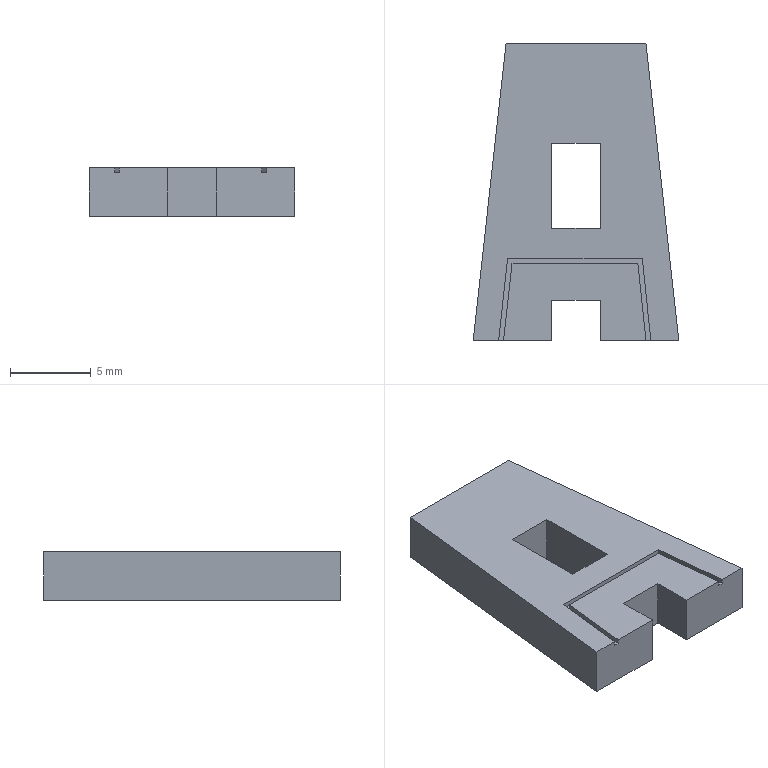Part | SolidWorks | features BaseBody 1 | 1 solid | 22 faces | box 12.712 x 18.351 x 3 mm | volume 516.696 mm3 | plane 21 | spline 1
STEP:
#1=CARTESIAN_POINT('',(103.606,-126.263,1.5));
#2=VERTEX_POINT('',#1);
#3=CARTESIAN_POINT('',(111.929,-126.263,1.5));
#4=VERTEX_POINT('',#3);
#5=CARTESIAN_POINT('',(103.606,-126.263,1.5));
#6=DIRECTION('',(1.,0.,0.));
#7=VECTOR('',#6,1000.);
#8=LINE('',#5,#7);
#9=EDGE_CURVE('',#2,#4,#8,.T.);
#10=ORIENTED_EDGE('',*,*,#9,.F.);
#11=CARTESIAN_POINT('',(103.606,-126.263,1.2));
#12=VERTEX_POINT('',#11);
#13=CARTESIAN_POINT('',(103.606,-126.263,1.2));
#14=DIRECTION('',(0.,0.,1.));
#15=VECTOR('',#14,1000.);
#16=LINE('',#13,#15);
#17=EDGE_CURVE('',#12,#2,#16,.T.);
#18=ORIENTED_EDGE('',*,*,#17,.F.);
#19=CARTESIAN_POINT('',(111.929,-126.263,1.2));
#20=VERTEX_POINT('',#19);
#21=CARTESIAN_POINT('',(103.606,-126.263,1.2));
#22=DIRECTION('',(1.,0.,0.));
#23=VECTOR('',#22,1000.);
#24=LINE('',#21,#23);
#25=EDGE_CURVE('',#12,#20,#24,.T.);
#26=ORIENTED_EDGE('',*,*,#25,.T.);
#27=CARTESIAN_POINT('',(111.929,-126.263,1.2));
#28=DIRECTION('',(0.,0.,1.));
#29=VECTOR('',#28,1000.);
#30=LINE('',#27,#29);
#31=EDGE_CURVE('',#20,#4,#30,.T.);
#32=ORIENTED_EDGE('',*,*,#31,.T.);
#33=EDGE_LOOP('',(#10,#18,#26,#32));
#34=FACE_OUTER_BOUND('',#33,.T.);
#35=CARTESIAN_POINT('',(103.606,-126.263,1.2));
#36=DIRECTION('',(0.,-1.,0.));
#37=DIRECTION('',(0.,0.,-1.));
#38=AXIS2_PLACEMENT_3D('',#35,#36,#37);
#39=PLANE('',#38);
#40=ADVANCED_FACE('',(#34),#39,.T.);
#41=CARTESIAN_POINT('',(103.875,-126.563,1.5));
#42=VERTEX_POINT('',#41);
#43=CARTESIAN_POINT('',(111.659,-126.563,1.5));
#44=VERTEX_POINT('',#43);
#45=CARTESIAN_POINT('',(103.606,-126.563,1.5));
#46=DIRECTION('',(1.,0.,0.));
#47=VECTOR('',#46,1000.);
#48=LINE('',#45,#47);
#49=EDGE_CURVE('',#42,#44,#48,.T.);
#50=ORIENTED_EDGE('',*,*,#49,.T.);
#51=CARTESIAN_POINT('',(111.659,-126.563,1.2));
#52=VERTEX_POINT('',#51);
#53=CARTESIAN_POINT('',(111.659,-126.563,1.2));
#54=DIRECTION('',(0.,0.,1.));
#55=VECTOR('',#54,1000.);
#56=LINE('',#53,#55);
#57=EDGE_CURVE('',#52,#44,#56,.T.);
#58=ORIENTED_EDGE('',*,*,#57,.F.);
#59=CARTESIAN_POINT('',(103.875,-126.563,1.2));
#60=VERTEX_POINT('',#59);
#61=CARTESIAN_POINT('',(103.606,-126.563,1.2));
#62=DIRECTION('',(1.,0.,0.));
#63=VECTOR('',#62,1000.);
#64=LINE('',#61,#63);
#65=EDGE_CURVE('',#60,#52,#64,.T.);
#66=ORIENTED_EDGE('',*,*,#65,.F.);
#67=CARTESIAN_POINT('',(103.875,-126.563,1.2));
#68=DIRECTION('',(0.,0.,1.));
#69=VECTOR('',#68,1000.);
#70=LINE('',#67,#69);
#71=EDGE_CURVE('',#60,#42,#70,.T.);
#72=ORIENTED_EDGE('',*,*,#71,.T.);
#73=EDGE_LOOP('',(#50,#58,#66,#72));
#74=FACE_OUTER_BOUND('',#73,.T.);
#75=CARTESIAN_POINT('',(103.606,-126.563,1.2));
#76=DIRECTION('',(0.,-1.,0.));
#77=DIRECTION('',(0.,0.,-1.));
#78=AXIS2_PLACEMENT_3D('',#75,#76,#77);
#79=PLANE('',#78);
#80=ADVANCED_FACE('',(#74),#79,.F.);
#81=CARTESIAN_POINT('',(112.461,-131.327,1.2));
#82=VERTEX_POINT('',#81);
#83=CARTESIAN_POINT('',(112.461,-131.327,1.5));
#84=VERTEX_POINT('',#83);
#85=CARTESIAN_POINT('',(112.461,-131.327,-1.5));
#86=DIRECTION('',(0.,0.,1.));
#87=VECTOR('',#86,1000.);
#88=LINE('',#85,#87);
#89=EDGE_CURVE('',#82,#84,#88,.T.);
#90=ORIENTED_EDGE('',*,*,#89,.T.);
#91=CARTESIAN_POINT('',(111.929,-126.263,1.5));
#92=DIRECTION('',(0.1043,-0.9945,0.));
#93=VECTOR('',#92,1000.);
#94=LINE('',#91,#93);
#95=EDGE_CURVE('',#4,#84,#94,.T.);
#96=ORIENTED_EDGE('',*,*,#95,.F.);
#97=ORIENTED_EDGE('',*,*,#31,.F.);
#98=CARTESIAN_POINT('',(111.929,-126.263,1.2));
#99=DIRECTION('',(0.1043,-0.9945,0.));
#100=VECTOR('',#99,1000.);
#101=LINE('',#98,#100);
#102=EDGE_CURVE('',#20,#82,#101,.T.);
#103=ORIENTED_EDGE('',*,*,#102,.T.);
#104=EDGE_LOOP('',(#90,#96,#97,#103));
#105=FACE_OUTER_BOUND('',#104,.T.);
#106=CARTESIAN_POINT('',(111.929,-126.263,1.2));
#107=DIRECTION('',(-0.9945,-0.1043,0.));
#108=DIRECTION('',(-0.1043,0.9945,0.));
#109=AXIS2_PLACEMENT_3D('',#106,#107,#108);
#110=PLANE('',#109);
#111=ADVANCED_FACE('',(#105),#110,.T.);
#112=CARTESIAN_POINT('',(103.046,-131.327,1.5));
#113=VERTEX_POINT('',#112);
#114=CARTESIAN_POINT('',(103.046,-131.327,1.2));
#115=VERTEX_POINT('',#114);
#116=CARTESIAN_POINT('',(103.046,-131.327,-1.5));
#117=DIRECTION('',(0.,0.,-1.));
#118=VECTOR('',#117,1000.);
#119=LINE('',#116,#118);
#120=EDGE_CURVE('',#113,#115,#119,.T.);
#121=ORIENTED_EDGE('',*,*,#120,.T.);
#122=CARTESIAN_POINT('',(102.875,-132.867,1.2));
#123=DIRECTION('',(0.1101,0.9939,0.));
#124=VECTOR('',#123,1000.);
#125=LINE('',#122,#124);
#126=EDGE_CURVE('',#115,#12,#125,.T.);
#127=ORIENTED_EDGE('',*,*,#126,.T.);
#128=ORIENTED_EDGE('',*,*,#17,.T.);
#129=CARTESIAN_POINT('',(116.164,-12.864,1.5));
#130=DIRECTION('',(0.1101,0.9939,0.));
#131=VECTOR('',#130,1000.);
#132=LINE('',#129,#131);
#133=EDGE_CURVE('',#113,#2,#132,.T.);
#134=ORIENTED_EDGE('',*,*,#133,.F.);
#135=EDGE_LOOP('',(#121,#127,#128,#134));
#136=FACE_OUTER_BOUND('',#135,.T.);
#137=CARTESIAN_POINT('',(102.875,-132.867,1.2));
#138=DIRECTION('',(0.9939,-0.1101,0.));
#139=DIRECTION('',(0.,0.,-1.));
#140=AXIS2_PLACEMENT_3D('',#137,#138,#139);
#141=PLANE('',#140);
#142=ADVANCED_FACE('',(#136),#141,.T.);
#143=CARTESIAN_POINT('',(103.347,-131.327,1.5));
#144=VERTEX_POINT('',#143);
#145=CARTESIAN_POINT('',(116.462,-12.897,1.5));
#146=DIRECTION('',(0.1101,0.9939,0.));
#147=VECTOR('',#146,1000.);
#148=LINE('',#145,#147);
#149=EDGE_CURVE('',#144,#42,#148,.T.);
#150=ORIENTED_EDGE('',*,*,#149,.T.);
#151=ORIENTED_EDGE('',*,*,#71,.F.);
#152=CARTESIAN_POINT('',(103.347,-131.327,1.2));
#153=VERTEX_POINT('',#152);
#154=CARTESIAN_POINT('',(103.173,-132.9,1.2));
#155=DIRECTION('',(0.1101,0.9939,0.));
#156=VECTOR('',#155,1000.);
#157=LINE('',#154,#156);
#158=EDGE_CURVE('',#153,#60,#157,.T.);
#159=ORIENTED_EDGE('',*,*,#158,.F.);
#160=CARTESIAN_POINT('',(103.347,-131.327,-1.5));
#161=DIRECTION('',(0.,0.,-1.));
#162=VECTOR('',#161,1000.);
#163=LINE('',#160,#162);
#164=EDGE_CURVE('',#144,#153,#163,.T.);
#165=ORIENTED_EDGE('',*,*,#164,.F.);
#166=EDGE_LOOP('',(#150,#151,#159,#165));
#167=FACE_OUTER_BOUND('',#166,.T.);
#168=CARTESIAN_POINT('',(103.173,-132.9,1.2));
#169=DIRECTION('',(0.9939,-0.1101,0.));
#170=DIRECTION('',(0.,0.,-1.));
#171=AXIS2_PLACEMENT_3D('',#168,#169,#170);
#172=PLANE('',#171);
#173=ADVANCED_FACE('',(#167),#172,.F.);
#174=CARTESIAN_POINT('',(112.159,-131.327,1.2));
#175=VERTEX_POINT('',#174);
#176=CARTESIAN_POINT('',(111.631,-126.294,1.2));
#177=DIRECTION('',(0.1043,-0.9945,0.));
#178=VECTOR('',#177,1000.);
#179=LINE('',#176,#178);
#180=EDGE_CURVE('',#52,#175,#179,.T.);
#181=ORIENTED_EDGE('',*,*,#180,.F.);
#182=ORIENTED_EDGE('',*,*,#57,.T.);
#183=CARTESIAN_POINT('',(112.159,-131.327,1.5));
#184=VERTEX_POINT('',#183);
#185=CARTESIAN_POINT('',(111.631,-126.294,1.5));
#186=DIRECTION('',(0.1043,-0.9945,0.));
#187=VECTOR('',#186,1000.);
#188=LINE('',#185,#187);
#189=EDGE_CURVE('',#44,#184,#188,.T.);
#190=ORIENTED_EDGE('',*,*,#189,.T.);
#191=CARTESIAN_POINT('',(112.159,-131.327,-1.5));
#192=DIRECTION('',(0.,0.,1.));
#193=VECTOR('',#192,1000.);
#194=LINE('',#191,#193);
#195=EDGE_CURVE('',#175,#184,#194,.T.);
#196=ORIENTED_EDGE('',*,*,#195,.F.);
#197=EDGE_LOOP('',(#181,#182,#190,#196));
#198=FACE_OUTER_BOUND('',#197,.T.);
#199=CARTESIAN_POINT('',(111.631,-126.294,1.2));
#200=DIRECTION('',(-0.9945,-0.1043,0.));
#201=DIRECTION('',(-0.1043,0.9945,0.));
#202=AXIS2_PLACEMENT_3D('',#199,#200,#201);
#203=PLANE('',#202);
#204=ADVANCED_FACE('',(#198),#203,.F.);
#205=ORIENTED_EDGE('',*,*,#102,.F.);
#206=ORIENTED_EDGE('',*,*,#25,.F.);
#207=ORIENTED_EDGE('',*,*,#126,.F.);
#208=CARTESIAN_POINT('',(0.,-131.327,1.2));
#209=DIRECTION('',(-1.,0.,0.));
#210=VECTOR('',#209,1000.);
#211=LINE('',#208,#210);
#212=EDGE_CURVE('',#153,#115,#211,.T.);
#213=ORIENTED_EDGE('',*,*,#212,.F.);
#214=ORIENTED_EDGE('',*,*,#158,.T.);
#215=ORIENTED_EDGE('',*,*,#65,.T.);
#216=ORIENTED_EDGE('',*,*,#180,.T.);
#217=CARTESIAN_POINT('',(0.,-131.327,1.2));
#218=DIRECTION('',(-1.,0.,0.));
#219=VECTOR('',#218,1000.);
#220=LINE('',#217,#219);
#221=EDGE_CURVE('',#82,#175,#220,.T.);
#222=ORIENTED_EDGE('',*,*,#221,.F.);
#223=EDGE_LOOP('',(#205,#206,#207,#213,#214,#215,#216,#222));
#224=FACE_OUTER_BOUND('',#223,.T.);
#225=CARTESIAN_POINT('',(0.,0.,1.2));
#226=DIRECTION('',(0.,0.,-1.));
#227=DIRECTION('',(0.,-1.,0.));
#228=AXIS2_PLACEMENT_3D('',#225,#226,#227);
#229=PLANE('',#228);
#230=ADVANCED_FACE('',(#224),#229,.F.);
#231=ORIENTED_EDGE('',*,*,#189,.F.);
#232=ORIENTED_EDGE('',*,*,#49,.F.);
#233=ORIENTED_EDGE('',*,*,#149,.F.);
#234=CARTESIAN_POINT('',(106.335,-131.327,1.5));
#235=VERTEX_POINT('',#234);
#236=CARTESIAN_POINT('',(0.,-131.327,1.5));
#237=DIRECTION('',(-1.,0.,0.));
#238=VECTOR('',#237,1000.);
#239=LINE('',#236,#238);
#240=EDGE_CURVE('',#235,#144,#239,.T.);
#241=ORIENTED_EDGE('',*,*,#240,.F.);
#242=CARTESIAN_POINT('',(106.335,-128.839,1.5));
#243=VERTEX_POINT('',#242);
#244=CARTESIAN_POINT('',(106.335,0.,1.5));
#245=DIRECTION('',(0.,-1.,0.));
#246=VECTOR('',#245,1000.);
#247=LINE('',#244,#246);
#248=EDGE_CURVE('',#243,#235,#247,.T.);
#249=ORIENTED_EDGE('',*,*,#248,.F.);
#250=CARTESIAN_POINT('',(109.33,-128.839,1.5));
#251=VERTEX_POINT('',#250);
#252=CARTESIAN_POINT('',(0.,-128.839,1.5));
#253=DIRECTION('',(-1.,0.,0.));
#254=VECTOR('',#253,1000.);
#255=LINE('',#252,#254);
#256=EDGE_CURVE('',#251,#243,#255,.T.);
#257=ORIENTED_EDGE('',*,*,#256,.F.);
#258=CARTESIAN_POINT('',(109.33,-131.327,1.5));
#259=VERTEX_POINT('',#258);
#260=CARTESIAN_POINT('',(109.33,0.,1.5));
#261=DIRECTION('',(0.,1.,0.));
#262=VECTOR('',#261,1000.);
#263=LINE('',#260,#262);
#264=EDGE_CURVE('',#259,#251,#263,.T.);
#265=ORIENTED_EDGE('',*,*,#264,.F.);
#266=CARTESIAN_POINT('',(0.,-131.327,1.5));
#267=DIRECTION('',(-1.,0.,0.));
#268=VECTOR('',#267,1000.);
#269=LINE('',#266,#268);
#270=EDGE_CURVE('',#184,#259,#269,.T.);
#271=ORIENTED_EDGE('',*,*,#270,.F.);
#272=EDGE_LOOP('',(#231,#232,#233,#241,#249,#257,#265,#271));
#273=FACE_OUTER_BOUND('',#272,.T.);
#274=CARTESIAN_POINT('',(0.,0.,1.5));
#275=DIRECTION('',(0.,0.,1.));
#276=DIRECTION('',(1.,0.,0.));
#277=AXIS2_PLACEMENT_3D('',#274,#275,#276);
#278=PLANE('',#277);
#279=ADVANCED_FACE('',(#273),#278,.T.);
#280=CARTESIAN_POINT('',(106.335,-119.133,-1.5));
#281=VERTEX_POINT('',#280);
#282=CARTESIAN_POINT('',(106.335,-124.395,-1.5));
#283=VERTEX_POINT('',#282);
#284=CARTESIAN_POINT('',(106.335,0.,-1.5));
#285=DIRECTION('',(0.,-1.,0.));
#286=VECTOR('',#285,1000.);
#287=LINE('',#284,#286);
#288=EDGE_CURVE('',#281,#283,#287,.T.);
#289=ORIENTED_EDGE('',*,*,#288,.T.);
#290=CARTESIAN_POINT('',(109.33,-124.395,-1.5));
#291=VERTEX_POINT('',#290);
#292=CARTESIAN_POINT('',(0.,-124.395,-1.5));
#293=DIRECTION('',(1.,0.,0.));
#294=VECTOR('',#293,1000.);
#295=LINE('',#292,#294);
#296=EDGE_CURVE('',#283,#291,#295,.T.);
#297=ORIENTED_EDGE('',*,*,#296,.T.);
#298=CARTESIAN_POINT('',(109.33,-119.133,-1.5));
#299=VERTEX_POINT('',#298);
#300=CARTESIAN_POINT('',(109.33,0.,-1.5));
#301=DIRECTION('',(0.,1.,0.));
#302=VECTOR('',#301,1000.);
#303=LINE('',#300,#302);
#304=EDGE_CURVE('',#291,#299,#303,.T.);
#305=ORIENTED_EDGE('',*,*,#304,.T.);
#306=CARTESIAN_POINT('',(0.,-119.133,-1.5));
#307=DIRECTION('',(-1.,0.,0.));
#308=VECTOR('',#307,1000.);
#309=LINE('',#306,#308);
#310=EDGE_CURVE('',#299,#281,#309,.T.);
#311=ORIENTED_EDGE('',*,*,#310,.T.);
#312=EDGE_LOOP('',(#289,#297,#305,#311));
#313=FACE_BOUND('',#312,.T.);
#314=CARTESIAN_POINT('',(101.476,-131.327,-1.5));
#315=VERTEX_POINT('',#314);
#316=CARTESIAN_POINT('',(103.509,-112.976,-1.5));
#317=VERTEX_POINT('',#316);
#318=CARTESIAN_POINT('',(101.476,-131.327,-1.5));
#319=CARTESIAN_POINT('',(102.154,-125.21,-1.5));
#320=CARTESIAN_POINT('',(102.831,-119.094,-1.5));
#321=CARTESIAN_POINT('',(103.509,-112.976,-1.5));
#322=B_SPLINE_CURVE_WITH_KNOTS('',3,(#318,#319,#320,#321),.UNSPECIFIED.,.F.,.F.,(4,4),(0.06667,0.1333),.UNSPECIFIED.);
#323=EDGE_CURVE('',#315,#317,#322,.T.);
#324=ORIENTED_EDGE('',*,*,#323,.T.);
#325=CARTESIAN_POINT('',(112.156,-112.976,-1.5));
#326=VERTEX_POINT('',#325);
#327=CARTESIAN_POINT('',(0.,-112.976,-1.5));
#328=DIRECTION('',(1.,0.,0.));
#329=VECTOR('',#328,1000.);
#330=LINE('',#327,#329);
#331=EDGE_CURVE('',#317,#326,#330,.T.);
#332=ORIENTED_EDGE('',*,*,#331,.T.);
#333=CARTESIAN_POINT('',(114.188,-131.327,-1.5));
#334=VERTEX_POINT('',#333);
#335=CARTESIAN_POINT('',(98.438,10.901,-1.5));
#336=DIRECTION('',(0.1101,-0.9939,0.));
#337=VECTOR('',#336,1000.);
#338=LINE('',#335,#337);
#339=EDGE_CURVE('',#326,#334,#338,.T.);
#340=ORIENTED_EDGE('',*,*,#339,.T.);
#341=CARTESIAN_POINT('',(109.33,-131.327,-1.5));
#342=VERTEX_POINT('',#341);
#343=CARTESIAN_POINT('',(0.,-131.327,-1.5));
#344=DIRECTION('',(-1.,0.,0.));
#345=VECTOR('',#344,1000.);
#346=LINE('',#343,#345);
#347=EDGE_CURVE('',#334,#342,#346,.T.);
#348=ORIENTED_EDGE('',*,*,#347,.T.);
#349=CARTESIAN_POINT('',(109.33,-128.839,-1.5));
#350=VERTEX_POINT('',#349);
#351=CARTESIAN_POINT('',(109.33,0.,-1.5));
#352=DIRECTION('',(0.,1.,0.));
#353=VECTOR('',#352,1000.);
#354=LINE('',#351,#353);
#355=EDGE_CURVE('',#342,#350,#354,.T.);
#356=ORIENTED_EDGE('',*,*,#355,.T.);
#357=CARTESIAN_POINT('',(106.335,-128.839,-1.5));
#358=VERTEX_POINT('',#357);
#359=CARTESIAN_POINT('',(0.,-128.839,-1.5));
#360=DIRECTION('',(-1.,0.,0.));
#361=VECTOR('',#360,1000.);
#362=LINE('',#359,#361);
#363=EDGE_CURVE('',#350,#358,#362,.T.);
#364=ORIENTED_EDGE('',*,*,#363,.T.);
#365=CARTESIAN_POINT('',(106.335,-131.327,-1.5));
#366=VERTEX_POINT('',#365);
#367=CARTESIAN_POINT('',(106.335,0.,-1.5));
#368=DIRECTION('',(0.,-1.,0.));
#369=VECTOR('',#368,1000.);
#370=LINE('',#367,#369);
#371=EDGE_CURVE('',#358,#366,#370,.T.);
#372=ORIENTED_EDGE('',*,*,#371,.T.);
#373=CARTESIAN_POINT('',(0.,-131.327,-1.5));
#374=DIRECTION('',(-1.,0.,0.));
#375=VECTOR('',#374,1000.);
#376=LINE('',#373,#375);
#377=EDGE_CURVE('',#366,#315,#376,.T.);
#378=ORIENTED_EDGE('',*,*,#377,.T.);
#379=EDGE_LOOP('',(#324,#332,#340,#348,#356,#364,#372,#378));
#380=FACE_OUTER_BOUND('',#379,.T.);
#381=CARTESIAN_POINT('',(0.,0.,-1.5));
#382=DIRECTION('',(0.,0.,1.));
#383=DIRECTION('',(1.,0.,0.));
#384=AXIS2_PLACEMENT_3D('',#381,#382,#383);
#385=PLANE('',#384);
#386=ADVANCED_FACE('',(#313,#380),#385,.F.);
#387=CARTESIAN_POINT('',(109.33,-119.133,1.5));
#388=VERTEX_POINT('',#387);
#389=CARTESIAN_POINT('',(106.335,-119.133,1.5));
#390=VERTEX_POINT('',#389);
#391=CARTESIAN_POINT('',(0.,-119.133,1.5));
#392=DIRECTION('',(-1.,0.,0.));
#393=VECTOR('',#392,1000.);
#394=LINE('',#391,#393);
#395=EDGE_CURVE('',#388,#390,#394,.T.);
#396=ORIENTED_EDGE('',*,*,#395,.T.);
#397=CARTESIAN_POINT('',(106.335,-119.133,-1.5));
#398=DIRECTION('',(0.,0.,1.));
#399=VECTOR('',#398,1000.);
#400=LINE('',#397,#399);
#401=EDGE_CURVE('',#281,#390,#400,.T.);
#402=ORIENTED_EDGE('',*,*,#401,.F.);
#403=ORIENTED_EDGE('',*,*,#310,.F.);
#404=CARTESIAN_POINT('',(109.33,-119.133,-1.5));
#405=DIRECTION('',(0.,0.,1.));
#406=VECTOR('',#405,1000.);
#407=LINE('',#404,#406);
#408=EDGE_CURVE('',#299,#388,#407,.T.);
#409=ORIENTED_EDGE('',*,*,#408,.T.);
#410=EDGE_LOOP('',(#396,#402,#403,#409));
#411=FACE_OUTER_BOUND('',#410,.T.);
#412=CARTESIAN_POINT('',(0.,-119.133,-1.5));
#413=DIRECTION('',(0.,1.,0.));
#414=DIRECTION('',(1.,0.,0.));
#415=AXIS2_PLACEMENT_3D('',#412,#413,#414);
#416=PLANE('',#415);
#417=ADVANCED_FACE('',(#411),#416,.F.);
#418=ORIENTED_EDGE('',*,*,#240,.T.);
#419=ORIENTED_EDGE('',*,*,#164,.T.);
#420=ORIENTED_EDGE('',*,*,#212,.T.);
#421=ORIENTED_EDGE('',*,*,#120,.F.);
#422=CARTESIAN_POINT('',(101.476,-131.327,1.5));
#423=VERTEX_POINT('',#422);
#424=CARTESIAN_POINT('',(0.,-131.327,1.5));
#425=DIRECTION('',(-1.,0.,0.));
#426=VECTOR('',#425,1000.);
#427=LINE('',#424,#426);
#428=EDGE_CURVE('',#113,#423,#427,.T.);
#429=ORIENTED_EDGE('',*,*,#428,.T.);
#430=CARTESIAN_POINT('',(101.476,-131.327,-1.5));
#431=DIRECTION('',(0.,0.,1.));
#432=VECTOR('',#431,1000.);
#433=LINE('',#430,#432);
#434=EDGE_CURVE('',#315,#423,#433,.T.);
#435=ORIENTED_EDGE('',*,*,#434,.F.);
#436=ORIENTED_EDGE('',*,*,#377,.F.);
#437=CARTESIAN_POINT('',(106.335,-131.327,-1.5));
#438=DIRECTION('',(0.,0.,1.));
#439=VECTOR('',#438,1000.);
#440=LINE('',#437,#439);
#441=EDGE_CURVE('',#366,#235,#440,.T.);
#442=ORIENTED_EDGE('',*,*,#441,.T.);
#443=EDGE_LOOP('',(#418,#419,#420,#421,#429,#435,#436,#442));
#444=FACE_OUTER_BOUND('',#443,.T.);
#445=CARTESIAN_POINT('',(0.,-131.327,-1.5));
#446=DIRECTION('',(0.,1.,0.));
#447=DIRECTION('',(1.,0.,0.));
#448=AXIS2_PLACEMENT_3D('',#445,#446,#447);
#449=PLANE('',#448);
#450=ADVANCED_FACE('',(#444),#449,.F.);
#451=ORIENTED_EDGE('',*,*,#248,.T.);
#452=ORIENTED_EDGE('',*,*,#441,.F.);
#453=ORIENTED_EDGE('',*,*,#371,.F.);
#454=CARTESIAN_POINT('',(106.335,-128.839,-1.5));
#455=DIRECTION('',(0.,0.,1.));
#456=VECTOR('',#455,1000.);
#457=LINE('',#454,#456);
#458=EDGE_CURVE('',#358,#243,#457,.T.);
#459=ORIENTED_EDGE('',*,*,#458,.T.);
#460=EDGE_LOOP('',(#451,#452,#453,#459));
#461=FACE_OUTER_BOUND('',#460,.T.);
#462=CARTESIAN_POINT('',(106.335,0.,-1.5));
#463=DIRECTION('',(-1.,0.,0.));
#464=DIRECTION('',(0.,0.,1.));
#465=AXIS2_PLACEMENT_3D('',#462,#463,#464);
#466=PLANE('',#465);
#467=ADVANCED_FACE('',(#461),#466,.F.);
#468=ORIENTED_EDGE('',*,*,#256,.T.);
#469=ORIENTED_EDGE('',*,*,#458,.F.);
#470=ORIENTED_EDGE('',*,*,#363,.F.);
#471=CARTESIAN_POINT('',(109.33,-128.839,-1.5));
#472=DIRECTION('',(0.,0.,1.));
#473=VECTOR('',#472,1000.);
#474=LINE('',#471,#473);
#475=EDGE_CURVE('',#350,#251,#474,.T.);
#476=ORIENTED_EDGE('',*,*,#475,.T.);
#477=EDGE_LOOP('',(#468,#469,#470,#476));
#478=FACE_OUTER_BOUND('',#477,.T.);
#479=CARTESIAN_POINT('',(0.,-128.839,-1.5));
#480=DIRECTION('',(0.,1.,0.));
#481=DIRECTION('',(1.,0.,0.));
#482=AXIS2_PLACEMENT_3D('',#479,#480,#481);
#483=PLANE('',#482);
#484=ADVANCED_FACE('',(#478),#483,.F.);
#485=ORIENTED_EDGE('',*,*,#264,.T.);
#486=ORIENTED_EDGE('',*,*,#475,.F.);
#487=ORIENTED_EDGE('',*,*,#355,.F.);
#488=CARTESIAN_POINT('',(109.33,-131.327,-1.5));
#489=DIRECTION('',(0.,0.,1.));
#490=VECTOR('',#489,1000.);
#491=LINE('',#488,#490);
#492=EDGE_CURVE('',#342,#259,#491,.T.);
#493=ORIENTED_EDGE('',*,*,#492,.T.);
#494=EDGE_LOOP('',(#485,#486,#487,#493));
#495=FACE_OUTER_BOUND('',#494,.T.);
#496=CARTESIAN_POINT('',(109.33,0.,-1.5));
#497=DIRECTION('',(1.,0.,0.));
#498=DIRECTION('',(0.,1.,0.));
#499=AXIS2_PLACEMENT_3D('',#496,#497,#498);
#500=PLANE('',#499);
#501=ADVANCED_FACE('',(#495),#500,.F.);
#502=ORIENTED_EDGE('',*,*,#221,.T.);
#503=ORIENTED_EDGE('',*,*,#195,.T.);
#504=ORIENTED_EDGE('',*,*,#270,.T.);
#505=ORIENTED_EDGE('',*,*,#492,.F.);
#506=ORIENTED_EDGE('',*,*,#347,.F.);
#507=CARTESIAN_POINT('',(114.188,-131.327,1.5));
#508=VERTEX_POINT('',#507);
#509=CARTESIAN_POINT('',(114.188,-131.327,-1.5));
#510=DIRECTION('',(0.,0.,1.));
#511=VECTOR('',#510,1000.);
#512=LINE('',#509,#511);
#513=EDGE_CURVE('',#334,#508,#512,.T.);
#514=ORIENTED_EDGE('',*,*,#513,.T.);
#515=CARTESIAN_POINT('',(0.,-131.327,1.5));
#516=DIRECTION('',(-1.,0.,0.));
#517=VECTOR('',#516,1000.);
#518=LINE('',#515,#517);
#519=EDGE_CURVE('',#508,#84,#518,.T.);
#520=ORIENTED_EDGE('',*,*,#519,.T.);
#521=ORIENTED_EDGE('',*,*,#89,.F.);
#522=EDGE_LOOP('',(#502,#503,#504,#505,#506,#514,#520,#521));
#523=FACE_OUTER_BOUND('',#522,.T.);
#524=CARTESIAN_POINT('',(0.,-131.327,-1.5));
#525=DIRECTION('',(0.,1.,0.));
#526=DIRECTION('',(1.,0.,0.));
#527=AXIS2_PLACEMENT_3D('',#524,#525,#526);
#528=PLANE('',#527);
#529=ADVANCED_FACE('',(#523),#528,.F.);
#530=CARTESIAN_POINT('',(112.156,-112.976,1.5));
#531=VERTEX_POINT('',#530);
#532=CARTESIAN_POINT('',(98.438,10.901,1.5));
#533=DIRECTION('',(0.1101,-0.9939,0.));
#534=VECTOR('',#533,1000.);
#535=LINE('',#532,#534);
#536=EDGE_CURVE('',#531,#508,#535,.T.);
#537=ORIENTED_EDGE('',*,*,#536,.T.);
#538=ORIENTED_EDGE('',*,*,#513,.F.);
#539=ORIENTED_EDGE('',*,*,#339,.F.);
#540=CARTESIAN_POINT('',(112.156,-112.976,-1.5));
#541=DIRECTION('',(0.,0.,1.));
#542=VECTOR('',#541,1000.);
#543=LINE('',#540,#542);
#544=EDGE_CURVE('',#326,#531,#543,.T.);
#545=ORIENTED_EDGE('',*,*,#544,.T.);
#546=EDGE_LOOP('',(#537,#538,#539,#545));
#547=FACE_OUTER_BOUND('',#546,.T.);
#548=CARTESIAN_POINT('',(98.438,10.901,-1.5));
#549=DIRECTION('',(-0.9939,-0.1101,0.));
#550=DIRECTION('',(-0.1101,0.9939,0.));
#551=AXIS2_PLACEMENT_3D('',#548,#549,#550);
#552=PLANE('',#551);
#553=ADVANCED_FACE('',(#547),#552,.F.);
#554=CARTESIAN_POINT('',(103.509,-112.976,1.5));
#555=VERTEX_POINT('',#554);
#556=CARTESIAN_POINT('',(0.,-112.976,1.5));
#557=DIRECTION('',(1.,0.,0.));
#558=VECTOR('',#557,1000.);
#559=LINE('',#556,#558);
#560=EDGE_CURVE('',#555,#531,#559,.T.);
#561=ORIENTED_EDGE('',*,*,#560,.T.);
#562=ORIENTED_EDGE('',*,*,#544,.F.);
#563=ORIENTED_EDGE('',*,*,#331,.F.);
#564=CARTESIAN_POINT('',(103.509,-112.976,-1.5));
#565=DIRECTION('',(0.,0.,1.));
#566=VECTOR('',#565,1000.);
#567=LINE('',#564,#566);
#568=EDGE_CURVE('',#317,#555,#567,.T.);
#569=ORIENTED_EDGE('',*,*,#568,.T.);
#570=EDGE_LOOP('',(#561,#562,#563,#569));
#571=FACE_OUTER_BOUND('',#570,.T.);
#572=CARTESIAN_POINT('',(0.,-112.976,-1.5));
#573=DIRECTION('',(0.,-1.,0.));
#574=DIRECTION('',(0.,0.,-1.));
#575=AXIS2_PLACEMENT_3D('',#572,#573,#574);
#576=PLANE('',#575);
#577=ADVANCED_FACE('',(#571),#576,.F.);
#578=CARTESIAN_POINT('',(101.476,-131.327,1.5));
#579=CARTESIAN_POINT('',(102.154,-125.21,1.5));
#580=CARTESIAN_POINT('',(102.831,-119.094,1.5));
#581=CARTESIAN_POINT('',(103.509,-112.976,1.5));
#582=B_SPLINE_CURVE_WITH_KNOTS('',3,(#578,#579,#580,#581),.UNSPECIFIED.,.F.,.F.,(4,4),(0.06667,0.1333),.UNSPECIFIED.);
#583=EDGE_CURVE('',#423,#555,#582,.T.);
#584=ORIENTED_EDGE('',*,*,#583,.T.);
#585=ORIENTED_EDGE('',*,*,#568,.F.);
#586=ORIENTED_EDGE('',*,*,#323,.F.);
#587=ORIENTED_EDGE('',*,*,#434,.T.);
#588=EDGE_LOOP('',(#584,#585,#586,#587));
#589=FACE_OUTER_BOUND('',#588,.T.);
#590=CARTESIAN_POINT('',(101.476,-131.327,-1.5));
#591=CARTESIAN_POINT('',(101.476,-131.327,1.5));
#592=CARTESIAN_POINT('',(102.154,-125.21,-1.5));
#593=CARTESIAN_POINT('',(102.154,-125.21,1.5));
#594=CARTESIAN_POINT('',(102.831,-119.094,-1.5));
#595=CARTESIAN_POINT('',(102.831,-119.094,1.5));
#596=CARTESIAN_POINT('',(103.509,-112.976,-1.5));
#597=CARTESIAN_POINT('',(103.509,-112.976,1.5));
#598=B_SPLINE_SURFACE_WITH_KNOTS('',3,1,((#590,#591),(#592,#593),(#594,#595),(#596,#597)),.UNSPECIFIED.,.F.,.F.,.F.,(4,4),(2,2),(0.06667,0.1333),(0.,1.),.UNSPECIFIED.);
#599=ADVANCED_FACE('',(#589),#598,.F.);
#600=CARTESIAN_POINT('',(109.33,-124.395,1.5));
#601=VERTEX_POINT('',#600);
#602=CARTESIAN_POINT('',(109.33,0.,1.5));
#603=DIRECTION('',(0.,1.,0.));
#604=VECTOR('',#603,1000.);
#605=LINE('',#602,#604);
#606=EDGE_CURVE('',#601,#388,#605,.T.);
#607=ORIENTED_EDGE('',*,*,#606,.T.);
#608=ORIENTED_EDGE('',*,*,#408,.F.);
#609=ORIENTED_EDGE('',*,*,#304,.F.);
#610=CARTESIAN_POINT('',(109.33,-124.395,-1.5));
#611=DIRECTION('',(0.,0.,1.));
#612=VECTOR('',#611,1000.);
#613=LINE('',#610,#612);
#614=EDGE_CURVE('',#291,#601,#613,.T.);
#615=ORIENTED_EDGE('',*,*,#614,.T.);
#616=EDGE_LOOP('',(#607,#608,#609,#615));
#617=FACE_OUTER_BOUND('',#616,.T.);
#618=CARTESIAN_POINT('',(109.33,0.,-1.5));
#619=DIRECTION('',(1.,0.,0.));
#620=DIRECTION('',(0.,1.,0.));
#621=AXIS2_PLACEMENT_3D('',#618,#619,#620);
#622=PLANE('',#621);
#623=ADVANCED_FACE('',(#617),#622,.F.);
#624=CARTESIAN_POINT('',(106.335,-124.395,1.5));
#625=VERTEX_POINT('',#624);
#626=CARTESIAN_POINT('',(0.,-124.395,1.5));
#627=DIRECTION('',(1.,0.,0.));
#628=VECTOR('',#627,1000.);
#629=LINE('',#626,#628);
#630=EDGE_CURVE('',#625,#601,#629,.T.);
#631=ORIENTED_EDGE('',*,*,#630,.T.);
#632=ORIENTED_EDGE('',*,*,#614,.F.);
#633=ORIENTED_EDGE('',*,*,#296,.F.);
#634=CARTESIAN_POINT('',(106.335,-124.395,-1.5));
#635=DIRECTION('',(0.,0.,1.));
#636=VECTOR('',#635,1000.);
#637=LINE('',#634,#636);
#638=EDGE_CURVE('',#283,#625,#637,.T.);
#639=ORIENTED_EDGE('',*,*,#638,.T.);
#640=EDGE_LOOP('',(#631,#632,#633,#639));
#641=FACE_OUTER_BOUND('',#640,.T.);
#642=CARTESIAN_POINT('',(0.,-124.395,-1.5));
#643=DIRECTION('',(0.,-1.,0.));
#644=DIRECTION('',(0.,0.,-1.));
#645=AXIS2_PLACEMENT_3D('',#642,#643,#644);
#646=PLANE('',#645);
#647=ADVANCED_FACE('',(#641),#646,.F.);
#648=CARTESIAN_POINT('',(106.335,0.,1.5));
#649=DIRECTION('',(0.,-1.,0.));
#650=VECTOR('',#649,1000.);
#651=LINE('',#648,#650);
#652=EDGE_CURVE('',#390,#625,#651,.T.);
#653=ORIENTED_EDGE('',*,*,#652,.T.);
#654=ORIENTED_EDGE('',*,*,#638,.F.);
#655=ORIENTED_EDGE('',*,*,#288,.F.);
#656=ORIENTED_EDGE('',*,*,#401,.T.);
#657=EDGE_LOOP('',(#653,#654,#655,#656));
#658=FACE_OUTER_BOUND('',#657,.T.);
#659=CARTESIAN_POINT('',(106.335,0.,-1.5));
#660=DIRECTION('',(-1.,0.,0.));
#661=DIRECTION('',(0.,0.,1.));
#662=AXIS2_PLACEMENT_3D('',#659,#660,#661);
#663=PLANE('',#662);
#664=ADVANCED_FACE('',(#658),#663,.F.);
#665=ORIENTED_EDGE('',*,*,#652,.F.);
#666=ORIENTED_EDGE('',*,*,#395,.F.);
#667=ORIENTED_EDGE('',*,*,#606,.F.);
#668=ORIENTED_EDGE('',*,*,#630,.F.);
#669=EDGE_LOOP('',(#665,#666,#667,#668));
#670=FACE_BOUND('',#669,.T.);
#671=ORIENTED_EDGE('',*,*,#428,.F.);
#672=ORIENTED_EDGE('',*,*,#133,.T.);
#673=ORIENTED_EDGE('',*,*,#9,.T.);
#674=ORIENTED_EDGE('',*,*,#95,.T.);
#675=ORIENTED_EDGE('',*,*,#519,.F.);
#676=ORIENTED_EDGE('',*,*,#536,.F.);
#677=ORIENTED_EDGE('',*,*,#560,.F.);
#678=ORIENTED_EDGE('',*,*,#583,.F.);
#679=EDGE_LOOP('',(#671,#672,#673,#674,#675,#676,#677,#678));
#680=FACE_OUTER_BOUND('',#679,.T.);
#681=CARTESIAN_POINT('',(0.,0.,1.5));
#682=DIRECTION('',(0.,0.,1.));
#683=DIRECTION('',(1.,0.,0.));
#684=AXIS2_PLACEMENT_3D('',#681,#682,#683);
#685=PLANE('',#684);
#686=ADVANCED_FACE('',(#670,#680),#685,.T.);
#687=CLOSED_SHELL('',(#40,#80,#111,#142,#173,#204,#230,#279,#386,#417,#450,#467,#484,#501,#529,#553,#577,#599,#623,#647,#664,#686));
#688=MANIFOLD_SOLID_BREP('',#687);
#689=CARTESIAN_POINT('',(0.,0.,0.));
#690=DIRECTION('',(0.,0.,1.));
#691=DIRECTION('',(1.,0.,0.));
#692=AXIS2_PLACEMENT_3D('',#689,#690,#691);
#693=(LENGTH_UNIT()NAMED_UNIT(*)SI_UNIT(.MILLI.,.METRE.));
#694=UNCERTAINTY_MEASURE_WITH_UNIT(LENGTH_MEASURE(0.00001),#693,'','');
#695=(NAMED_UNIT(*)PLANE_ANGLE_UNIT()SI_UNIT($,.RADIAN.));
#696=(NAMED_UNIT(*)SI_UNIT($,.STERADIAN.)SOLID_ANGLE_UNIT());
#697=(GEOMETRIC_REPRESENTATION_CONTEXT(3)GLOBAL_UNCERTAINTY_ASSIGNED_CONTEXT((#694))GLOBAL_UNIT_ASSIGNED_CONTEXT((#693,#695,#696))REPRESENTATION_CONTEXT('',''));
#698=ADVANCED_BREP_SHAPE_REPRESENTATION('',(#688,#692),#697);